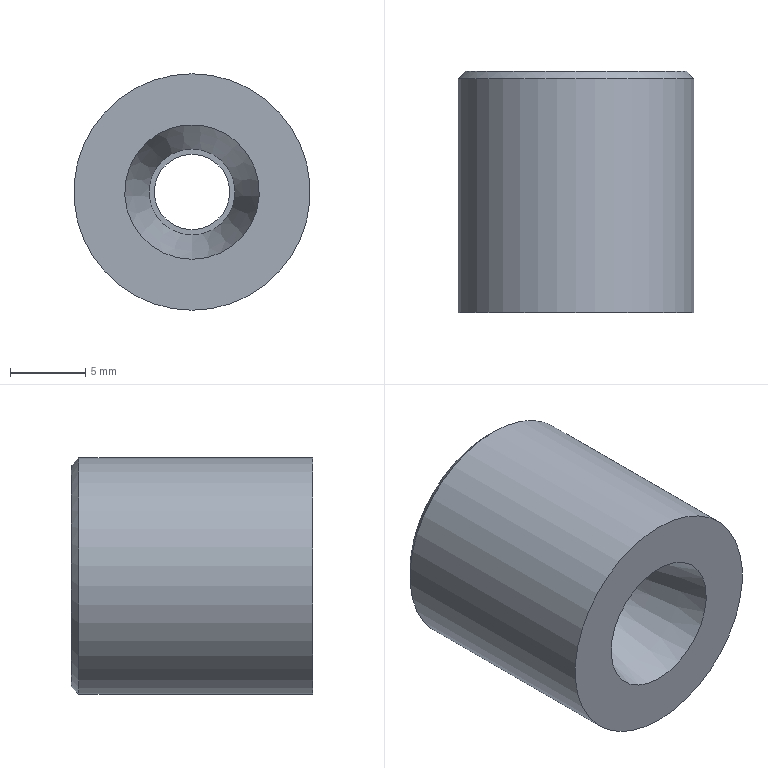Part | STEP file | Z05-16-2_id110_x_t | 1 solid | 7 faces | box 15.681 x 16 x 15.681 mm | volume 2631 mm3 | plane 3 | cylinder 2 | cone 2 | commonest cylinder face diameters 5 x1 15.681 x1
STEP:
#1=CARTESIAN_POINT('',(-140.,7.5,182.5));
#2=VERTEX_POINT('',#1);
#3=CARTESIAN_POINT('',(-140.,7.5,180.));
#4=DIRECTION('',(0.,1.,0.));
#5=DIRECTION('',(0.,0.,1.));
#6=AXIS2_PLACEMENT_3D('',#3,#4,#5);
#7=CIRCLE('',#6,2.5);
#8=EDGE_CURVE('',#2,#2,#7,.T.);
#9=ORIENTED_EDGE('',*,*,#8,.T.);
#10=EDGE_LOOP('',(#9));
#11=FACE_BOUND('',#10,.T.);
#12=CARTESIAN_POINT('',(-140.,7.5,177.144));
#13=VERTEX_POINT('',#12);
#14=CARTESIAN_POINT('',(-140.,7.5,180.));
#15=DIRECTION('',(0.,-1.,0.));
#16=DIRECTION('',(0.,0.,-1.));
#17=AXIS2_PLACEMENT_3D('',#14,#15,#16);
#18=CIRCLE('',#17,2.856);
#19=EDGE_CURVE('',#13,#13,#18,.T.);
#20=ORIENTED_EDGE('',*,*,#19,.T.);
#21=EDGE_LOOP('',(#20));
#22=FACE_BOUND('',#21,.T.);
#23=CARTESIAN_POINT('',(-140.,7.5,180.));
#24=DIRECTION('',(0.,1.,0.));
#25=DIRECTION('',(0.,0.,1.));
#26=AXIS2_PLACEMENT_3D('',#23,#24,#25);
#27=PLANE('',#26);
#28=ADVANCED_FACE('',(#11,#22),#27,.F.);
#29=ORIENTED_EDGE('',*,*,#8,.F.);
#30=EDGE_LOOP('',(#29));
#31=FACE_BOUND('',#30,.T.);
#32=CARTESIAN_POINT('',(-140.,17.5,182.5));
#33=VERTEX_POINT('',#32);
#34=CARTESIAN_POINT('',(-140.,17.5,180.));
#35=DIRECTION('',(0.,-1.,0.));
#36=DIRECTION('',(0.,0.,1.));
#37=AXIS2_PLACEMENT_3D('',#34,#35,#36);
#38=CIRCLE('',#37,2.5);
#39=EDGE_CURVE('',#33,#33,#38,.T.);
#40=ORIENTED_EDGE('',*,*,#39,.F.);
#41=EDGE_LOOP('',(#40));
#42=FACE_BOUND('',#41,.T.);
#43=CARTESIAN_POINT('',(-140.,18.3,180.));
#44=DIRECTION('',(0.,1.,0.));
#45=DIRECTION('',(0.,0.,1.));
#46=AXIS2_PLACEMENT_3D('',#43,#44,#45);
#47=CYLINDRICAL_SURFACE('',#46,2.5);
#48=ADVANCED_FACE('',(#31,#42),#47,.F.);
#49=CARTESIAN_POINT('',(-140.,1.5,175.536));
#50=VERTEX_POINT('',#49);
#51=CARTESIAN_POINT('',(-140.,1.5,180.));
#52=DIRECTION('',(0.,-1.,0.));
#53=DIRECTION('',(0.,0.,-1.));
#54=AXIS2_PLACEMENT_3D('',#51,#52,#53);
#55=CIRCLE('',#54,4.464);
#56=EDGE_CURVE('',#50,#50,#55,.T.);
#57=ORIENTED_EDGE('',*,*,#56,.T.);
#58=EDGE_LOOP('',(#57));
#59=FACE_BOUND('',#58,.T.);
#60=ORIENTED_EDGE('',*,*,#19,.F.);
#61=EDGE_LOOP('',(#60));
#62=FACE_BOUND('',#61,.T.);
#63=CARTESIAN_POINT('',(-140.,1.5,180.));
#64=DIRECTION('',(0.,-1.,0.));
#65=DIRECTION('',(0.,0.,-1.));
#66=AXIS2_PLACEMENT_3D('',#63,#64,#65);
#67=CONICAL_SURFACE('',#66,4.464,15.);
#68=ADVANCED_FACE('',(#59,#62),#67,.F.);
#69=ORIENTED_EDGE('',*,*,#39,.T.);
#70=EDGE_LOOP('',(#69));
#71=FACE_BOUND('',#70,.T.);
#72=CARTESIAN_POINT('',(-140.,17.5,172.659));
#73=VERTEX_POINT('',#72);
#74=CARTESIAN_POINT('',(-140.,17.5,180.));
#75=DIRECTION('',(0.,-1.,0.));
#76=DIRECTION('',(0.,0.,-1.));
#77=AXIS2_PLACEMENT_3D('',#74,#75,#76);
#78=CIRCLE('',#77,7.341);
#79=EDGE_CURVE('',#73,#73,#78,.T.);
#80=ORIENTED_EDGE('',*,*,#79,.F.);
#81=EDGE_LOOP('',(#80));
#82=FACE_BOUND('',#81,.T.);
#83=CARTESIAN_POINT('',(-140.,17.5,180.));
#84=DIRECTION('',(0.,1.,0.));
#85=DIRECTION('',(0.,0.,1.));
#86=AXIS2_PLACEMENT_3D('',#83,#84,#85);
#87=PLANE('',#86);
#88=ADVANCED_FACE('',(#71,#82),#87,.T.);
#89=ORIENTED_EDGE('',*,*,#56,.F.);
#90=EDGE_LOOP('',(#89));
#91=FACE_BOUND('',#90,.T.);
#92=CARTESIAN_POINT('',(-140.,1.5,187.841));
#93=VERTEX_POINT('',#92);
#94=CARTESIAN_POINT('',(-140.,1.5,180.));
#95=DIRECTION('',(0.,1.,0.));
#96=DIRECTION('',(0.,0.,1.));
#97=AXIS2_PLACEMENT_3D('',#94,#95,#96);
#98=CIRCLE('',#97,7.841);
#99=EDGE_CURVE('',#93,#93,#98,.T.);
#100=ORIENTED_EDGE('',*,*,#99,.F.);
#101=EDGE_LOOP('',(#100));
#102=FACE_BOUND('',#101,.T.);
#103=CARTESIAN_POINT('',(-140.,1.5,180.));
#104=DIRECTION('',(0.,1.,0.));
#105=DIRECTION('',(0.,0.,1.));
#106=AXIS2_PLACEMENT_3D('',#103,#104,#105);
#107=PLANE('',#106);
#108=ADVANCED_FACE('',(#91,#102),#107,.F.);
#109=ORIENTED_EDGE('',*,*,#79,.T.);
#110=EDGE_LOOP('',(#109));
#111=FACE_BOUND('',#110,.T.);
#112=CARTESIAN_POINT('',(-140.,17.,187.841));
#113=VERTEX_POINT('',#112);
#114=CARTESIAN_POINT('',(-140.,17.,180.));
#115=DIRECTION('',(0.,-1.,0.));
#116=DIRECTION('',(0.,0.,1.));
#117=AXIS2_PLACEMENT_3D('',#114,#115,#116);
#118=CIRCLE('',#117,7.841);
#119=EDGE_CURVE('',#113,#113,#118,.T.);
#120=ORIENTED_EDGE('',*,*,#119,.F.);
#121=EDGE_LOOP('',(#120));
#122=FACE_BOUND('',#121,.T.);
#123=CARTESIAN_POINT('',(-140.,17.,180.));
#124=DIRECTION('',(0.,-1.,0.));
#125=DIRECTION('',(0.,0.,-1.));
#126=AXIS2_PLACEMENT_3D('',#123,#124,#125);
#127=CONICAL_SURFACE('',#126,7.841,45.);
#128=ADVANCED_FACE('',(#111,#122),#127,.T.);
#129=ORIENTED_EDGE('',*,*,#119,.T.);
#130=EDGE_LOOP('',(#129));
#131=FACE_BOUND('',#130,.T.);
#132=ORIENTED_EDGE('',*,*,#99,.T.);
#133=EDGE_LOOP('',(#132));
#134=FACE_BOUND('',#133,.T.);
#135=CARTESIAN_POINT('',(-140.,18.3,180.));
#136=DIRECTION('',(0.,1.,0.));
#137=DIRECTION('',(0.,0.,1.));
#138=AXIS2_PLACEMENT_3D('',#135,#136,#137);
#139=CYLINDRICAL_SURFACE('',#138,7.841);
#140=ADVANCED_FACE('',(#131,#134),#139,.T.);
#141=CLOSED_SHELL('',(#28,#48,#68,#88,#108,#128,#140));
#142=MANIFOLD_SOLID_BREP('',#141);
#143=(LENGTH_UNIT()NAMED_UNIT(*)SI_UNIT(.MILLI.,.METRE.));
#144=UNCERTAINTY_MEASURE_WITH_UNIT(LENGTH_MEASURE(0.00002),#143,'','');
#145=(NAMED_UNIT(*)PLANE_ANGLE_UNIT()SI_UNIT($,.RADIAN.));
#146=PLANE_ANGLE_MEASURE_WITH_UNIT(PLANE_ANGLE_MEASURE(0.01745),#145);
#147=DIMENSIONAL_EXPONENTS(0.,0.,0.,0.,0.,0.,0.);
#148=(CONVERSION_BASED_UNIT('DEGREE',#146)NAMED_UNIT(#147)PLANE_ANGLE_UNIT());
#149=(NAMED_UNIT(*)SI_UNIT($,.STERADIAN.)SOLID_ANGLE_UNIT());
#150=(GEOMETRIC_REPRESENTATION_CONTEXT(3)GLOBAL_UNCERTAINTY_ASSIGNED_CONTEXT((#144))GLOBAL_UNIT_ASSIGNED_CONTEXT((#143,#148,#149))REPRESENTATION_CONTEXT('',''));
#151=ADVANCED_BREP_SHAPE_REPRESENTATION('',(#142),#150);